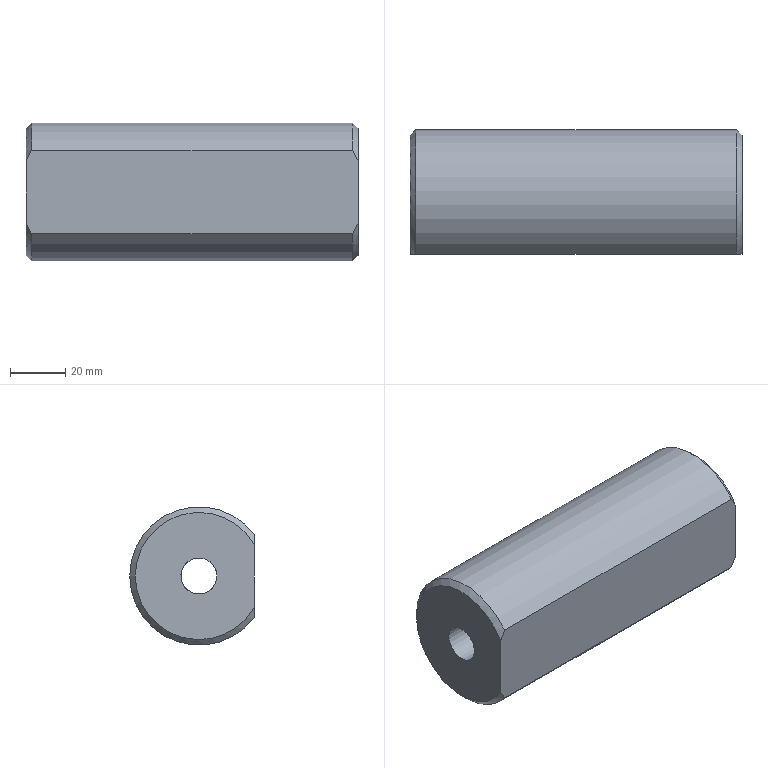Part | STEP file | solid 29 | 1 solid | 9 faces | box 120 x 45 x 50 mm | volume 204594 mm3 | plane 4 | cylinder 3 | cone 2 | commonest cylinder face diameters 13 x1 20 x1 50 x1